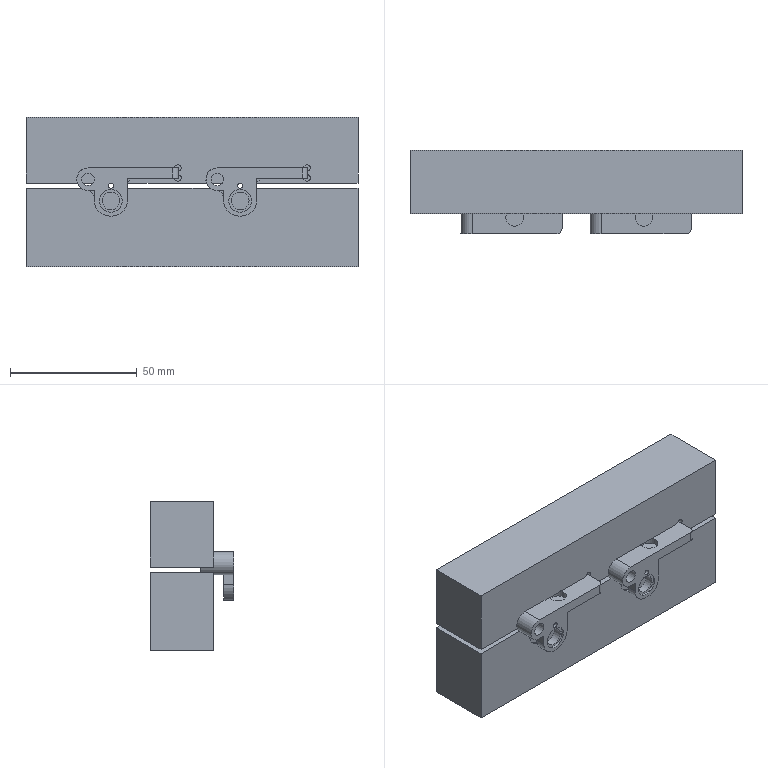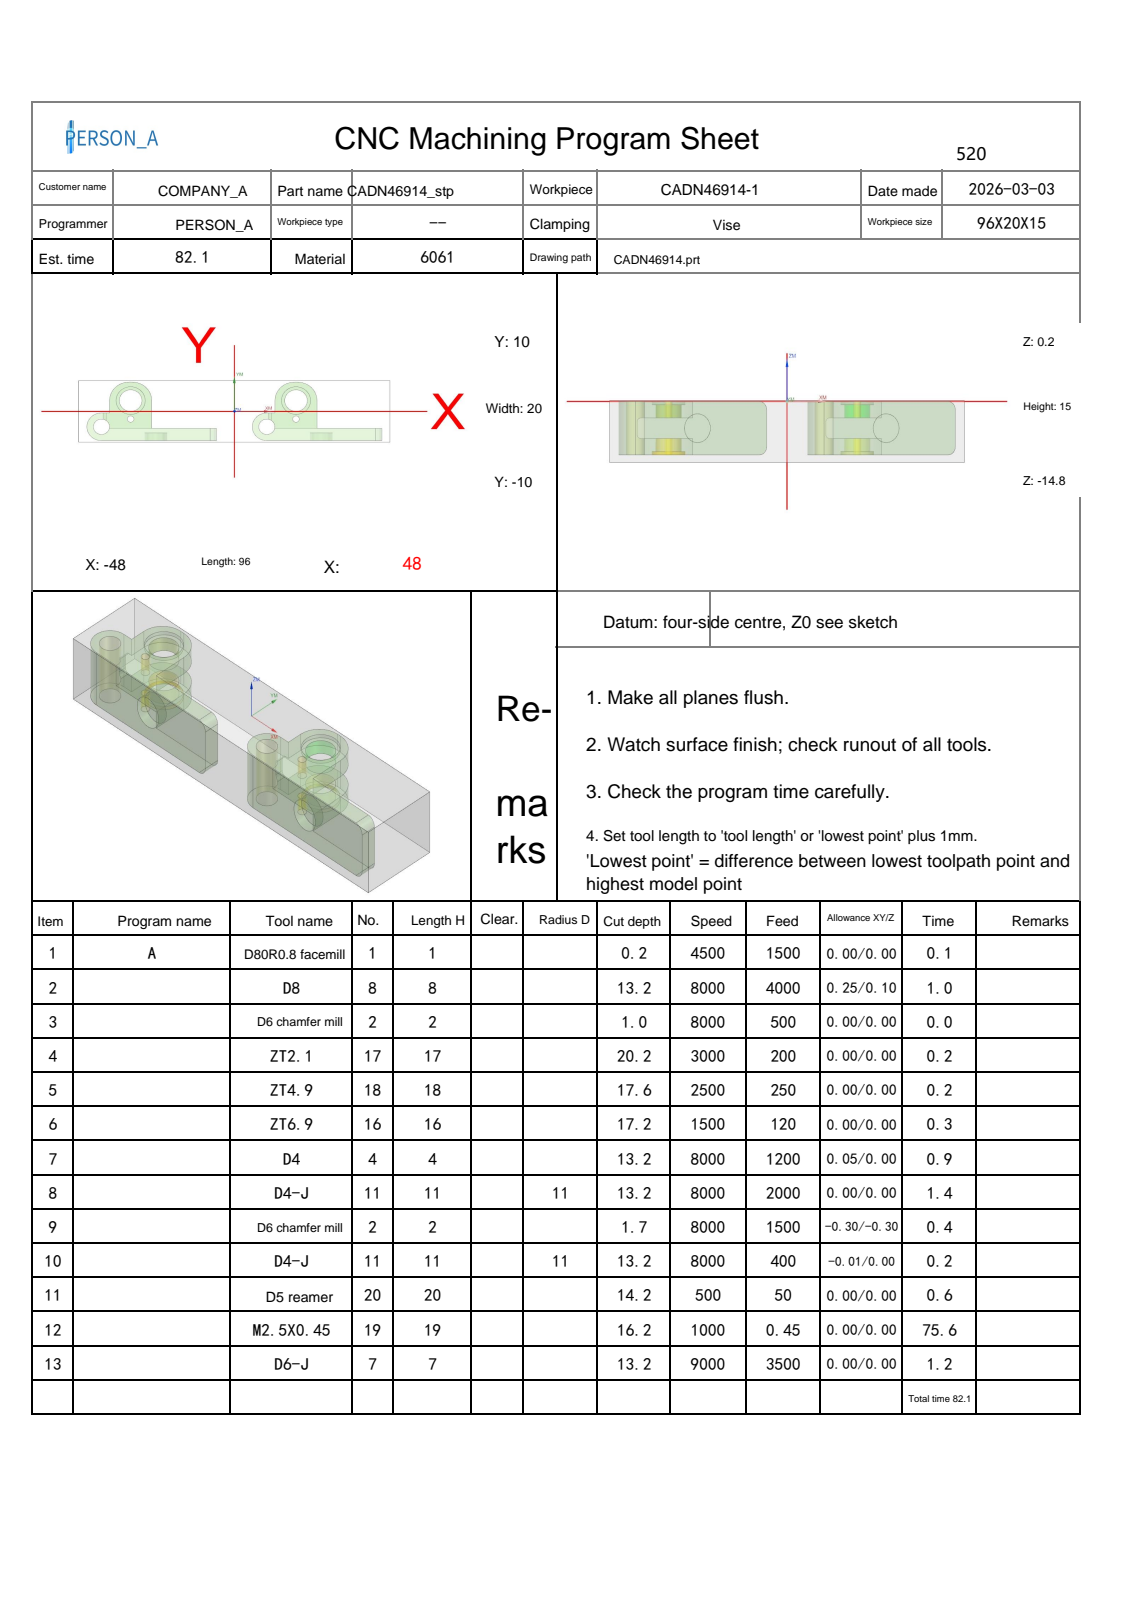NC program | NX | posted by the shop | part box 131 x 33 x 59 mm
Lines 1 to 1880 of 12027, first 1516 of 1878 lines:
%
O0001
(Machine time: 155.85 MIN)
(===Total Tool:11===)
(T1=D80R0.8 facemill D=80.  R=0.8  D-  H01 Z=-0.   )
(T8=D8      D=8.   R=0.   D-  H08 Z=-13.  )
(T2=D6 chamfer mill   D=6.   R=0.   D-  H02 Z=-1.5  )
(T17=ZT2.1  D=2.1  DR_a=118 D-  H17 Z=-20.  )
(T18=ZT4.9  D=4.9  DR_a=120 D-  H18 Z=-17.41)
(T16=ZT6.9  D=6.9  DR_a=120 D-  H16 Z=-17.  )
(T4=D4      D=4.   R=0.   D-  H04 Z=-13.  )
(T11=D4-J   D=4.   R=0.   D11 H11 Z=-13.  )
(T20=D5 reamer   D=5.   DR_a=180 D20 H20 Z=-14.  )
(T19=M2.5X0.45 D=2.05 DR_a=180 D-  H19 Z=-16.  )
(T7=D6-J    D=6.   R=0.   D7  H07 Z=-13.  )
G80 G90 G17 G49 G40
G91 G28 Z0
M01
N1 T01 M06
(D80R0.8 facemill  D=80. R=0.8 H=01 ce=0.00 di=0.00)
G00 G90 G54 X90.5 Y0.0 M03 S4500
G43 H01 Z50.
M08
Z2.
G01 Z0.0 F1500.
X85.5
X-85.5
X-90.5
Z2.
G00 Z50.
G91 G28 Z0.0
M05
M09
G91 G28 Z0.0
M01
N2 T08 M06
(D8  D=8. R=0. H=08 ce=0.25 di=0.10)
G00 G90 G54 X-31.173 Y-19.977 M03 S8000
G43 H08 Z50.
M08
Z-11.
G01 X-31.188 Y-19.879 Z-11.625 F4000.
X-31.204 Y-19.78 Z-11.872
X-31.219 Y-19.681 Z-12.054
X-31.234 Y-19.582 Z-12.2
X-31.249 Y-19.483 Z-12.323
X-31.265 Y-19.384 Z-12.428
X-31.28 Y-19.286 Z-12.52
X-31.295 Y-19.187 Z-12.6
X-31.31 Y-19.088 Z-12.67
X-31.326 Y-18.989 Z-12.732
X-31.341 Y-18.89 Z-12.786
X-31.356 Y-18.792 Z-12.833
X-31.372 Y-18.693 Z-12.874
X-31.387 Y-18.594 Z-12.908
X-31.402 Y-18.495 Z-12.936
X-31.417 Y-18.396 Z-12.96
X-31.433 Y-18.297 Z-12.977
X-31.448 Y-18.199 Z-12.99
X-31.463 Y-18.1 Z-12.997
X-31.478 Y-18.001 Z-13.
X-31.735 Y-16.34
G03 X-32.01 Y-16.017 I-.404 J-.066
X-35.519 Y-15.492 I-3.509 J-11.46
G01 X-35.593
G03 X-46.075 Y-15.381 I-10.483 J-496.321
G01 X-46.658 Y-15.382
G02 X-52.576 Y-10.87 I.001 J6.139
X-53.33 Y-5.373 I19.659 J5.497
G01 Y-5.3
G02 X-53.415 Y2.659 I373.963 J7.959
X-53.361 Y8.999 I374.048 J0.0
X-48.906 Y14.573 I6.101 J-.308
X-43.489 Y15.327 I5.418 J-19.103
G01 X-43.457 Y15.326
G02 X-34.113 Y15.4 I9.343 J-593.749
G01 X-33.498
X46.622 Y15.383
X46.677
G02 X52.525 Y11.02 I0.0 J-6.1
X53.318 Y5.638 I-18.167 J-5.425
X53.416 Y-2.714 I-356.305 J-8.352
X53.36 Y-9.02 I-356.403 J0.0
X49.041 Y-14.518 I-6.055 J.311
X43.556 Y-15.322 I-5.485 J18.317
G01 X43.54
G02 X34.581 Y-15.401 I-8.958 J507.142
G01 X33.58 Y-15.4
X-29.919 Y-15.386
G03 X-37.675 Y-14.858 I-12.074 J-120.03
G02 X-45.7 Y-14.758 I4.706 J700.045
X-51.384 Y-10.731 I.412 J6.606
X-52.632 Y-4.958 I14.903 J6.245
X-52.809 Y3.144 I185.372 J8.102
X-52.752 Y7.758 I185.549 J0.0
X-48.584 Y13.457 I6.632 J-.476
X-42.856 Y14.641 I6.186 J-15.48
X-34.645 Y14.811 I8.211 J-197.481
X-32.419 Y14.799 I0.0 J-197.652
G01 X45.361 Y14.777
G02 X51.385 Y10.727 I-.09 J-6.639
X52.62 Y5.134 I-14.626 J-6.161
X52.813 Y-3.12 I-176.538 J-8.254
X52.752 Y-7.761 I-176.731 J0.0
X48.731 Y-13.383 I-6.598 J.47
X43.199 Y-14.619 I-6.112 J14.36
X33.955 Y-14.822 I-9.244 J209.879
X30.842 Y-14.799 I0.0 J210.083
G01 X-28.817 Y-14.779
G03 X-38.511 Y-14.261 I-20.809 J-298.283
G01 X-38.8
G02 X-44.696 Y-14.139 I0.0 J142.819
X-50.671 Y-9.697 I.775 J7.281
X-51.996 Y-3.753 I15.854 J6.653
X-52.209 Y2.694 I97.671 J6.447
X-52.125 Y6.741 I97.884 J0.0
X-47.707 Y12.669 I7.254 J-.796
X-41.584 Y14.01 I6.722 J-16.049
X-31.957 Y14.222 I9.626 J-217.839
X-29.047 Y14.203 I0.0 J-218.052
G01 X44.038 Y14.178
G02 X50.697 Y9.638 I-.131 J-7.345
X52.001 Y3.691 I-16.077 J-6.639
X52.205 Y-2.78 I-102.305 J-6.471
X52.131 Y-6.684 I-102.51 J0.0
X48.862 Y-12.04 I-7.112 J.664
X47.625 Y-13.181 I-3.464 J2.517
X45.5 Y-13.75 I-2.305 J4.352
X36.302 Y-14.202 I-9.198 J93.33
X34.835 Y-14.191 I0.0 J93.782
G01 X-27.645 Y-14.182
G02 X-36.111 Y-13.75 I31.277 J696.242
X-38.142 Y-13.775 I-2.03 J82.632
X-42.93 Y-13.636 I0.0 J82.657
X-50.092 Y-8.528 I.327 J8.034
X-51.415 Y-2.034 I18.291 J7.107
X-51.579 Y2.607 I65.409 J4.64
X-51.514 Y5.521 I65.573 J0.0
X-46.754 Y11.985 I7.803 J-.761
X-40.64 Y13.371 I6.966 J-16.556
X-34.235 Y13.583 I6.881 J-110.809
X-31.707 Y13.747 I2.528 J-19.451
X-29.968 Y13.67 I0.0 J-19.614
G03 X-20.778 Y13.6 I9.191 J605.473
G01 X-20.602
X16.938
G02 X19.516 Y13.752 I2.578 J-21.824
X21.449 Y13.666 I0.0 J-21.976
G03 X34.707 Y13.576 I13.258 J972.338
X41.458 Y13.599 I0.0 J972.429
G02 X42.084 Y13.617 I.626 J-10.91
X45.763 Y12.979 I0.0 J-10.928
X50.312 Y7.97 I-3.406 J-7.663
X51.448 Y1.494 I-20.828 J-6.991
X51.582 Y-2.563 I-61.296 J-4.057
X51.507 Y-5.581 I-61.431 J0.0
X49.714 Y-9.906 I-8.423 J.958
X48.852 Y-12.053 I-3.864 J.305
G03 X49.706 Y-9.872 I-2.976 J2.423
X51.03 Y-2.986 I-17.238 J6.886
X51.026 Y-2.565 I-18.562 J0.0
X51.047 Y-1.316 I-37.014 J1.249
X50.415 Y5.496 I-37.035 J0.0
X47.669 Y10.726 I-9.664 J-1.738
X42.536 Y12.852 I-5.851 J-6.867
X36.521 Y13.127 I-6.015 J-65.771
X35.284 Y13.115 I0.0 J-66.046
G02 X32.132 Y13.106 I-3.152 J555.883
X22.821 Y13.184 I0.0 J555.892
G03 X20.121 Y13.728 I-3.812 J-11.937
G02 X23.466 Y12.961 I-1.169 J-12.769
G03 X28.086 Y12.551 I4.62 J25.827
X28.536 Y12.555 I0.0 J26.237
G01 X28.787
G02 X39.905 Y12.42 I0.0 J-457.028
X44.815 Y11.431 I-.102 J-13.192
X49.287 Y6.166 I-3.935 J-7.873
X50.357 Y-.852 I-22.46 J-7.018
G01 Y-.865
G02 X50.391 Y-2.083 I-22.145 J-1.218
X49.75 Y-7.376 I-22.178 J0.0
X49.771 Y-8.246 I-17.879 J-.87
X49.687 Y-9.978 I-17.9 J0.0
G03 X49.771 Y-8.246 I-17.816 J1.731
X49.75 Y-7.376 I-17.9 J0.0
G01 X49.856 Y-1.619
G03 X49.859 Y-1.299 I-23.764 J.32
X48.904 Y5.37 I-23.766 J0.0
X42.148 Y11.442 I-8.36 J-2.507
X35.985 Y12.016 I-6.163 J-32.851
X35.464 Y12.012 I0.0 J-33.424
G02 X34.223 Y12.007 I-1.241 J169.499
X25.721 Y12.22 I0.0 J169.503
X24.568 Y12.388 I.85 J9.879
G03 X22.994 Y13.11 I-4.602 J-7.962
G02 X25.036 Y12.15 I-7.062 J-17.675
G03 X29.128 Y11.549 I4.183 J14.252
G02 X38.003 Y11.306 I-17.561 J-803.143
X43.381 Y10.202 I-.355 J-15.383
X48.148 Y4.731 I-3.889 J-8.2
X49.199 Y-2.119 I-21.803 J-6.85
X49.192 Y-2.663 I-22.854 J0.0
G01 X49.213 Y-3.454
G02 X49.75 Y-5.502 I-4.134 J-2.177
G01 Y-6.282
G03 X49.77 Y-5.816 I-5.325 J.466
X49.181 Y-3.375 I-5.345 J0.0
G02 X48.598 Y.165 I21.975 J5.431
G03 X46.88 Y5.94 I-15.451 J-1.456
X40.825 Y10.245 I-7.949 J-4.77
X34.296 Y10.925 I-6.529 J-31.005
G01 X34.213
X34.11
G02 X26.951 Y11.311 I0.0 J66.524
G01 X25.816 Y11.561
X24.666 Y12.323
G03 X26.591 Y11.159 I6.474 J8.534
X31.008 Y10.477 I4.736 J16.027
G02 X38.201 Y10.026 I-2.816 J-102.487
X43.722 Y8.015 I-1.074 J-11.533
X47.372 Y2.285 I-6.546 J-8.197
X48.355 Y-2.273 I-119.995 J-28.268
G01 X49.181 Y-3.375
G02 X48.159 Y-1.981 I6.846 J6.089
X46.987 Y1.793 I41.138 J14.841
G03 X43.528 Y7.177 I-10.292 J-2.81
X37.723 Y9.457 I-7.253 J-9.935
X30.746 Y10.029 I-11.086 J-92.462
G02 X26.669 Y10.791 I.523 J14.084
G01 X25.902 Y11.504
G03 X27.46 Y10.29 I3.757 J3.213
X31.921 Y9.416 I5.217 J14.815
G02 X38.256 Y8.659 I-2.824 J-50.506
X45.91 Y2.299 I-1.91 J-10.083
G03 X47.389 Y-1.48 I172.833 J65.472
X47.654 Y-1.842 I1.213 J.612
G01 X48.505 Y-2.495
G02 X47.254 Y-1.443 I3.601 J5.554
X45.612 Y1.782 I20.773 J12.61
G03 X37.889 Y8.06 I-9.997 J-4.408
X31.486 Y8.985 I-10.718 J-51.591
G02 X27.474 Y9.945 I1.011 J13.082
G01 X26.707 Y10.733
X27.657 Y9.749
G03 X30.84 Y8.612 I4.25 J6.871
G02 X36.544 Y7.677 I-31.05 J-207.346
X42.97 Y4.191 I-2.042 J-11.431
X45.724 Y-.006 I-17.256 J-14.325
G03 X46.785 Y-1.471 I4.78 J2.344
G01 X47.625 Y-1.819
G02 X45.51 Y-.187 I.987 J3.466
G03 X42.711 Y3.573 I-27.418 J-17.488
X36.083 Y7.146 I-9.148 J-9.038
X30.559 Y8.223 I-147.226 J-740.215
G02 X27.945 Y9.244 I1.369 J7.362
G01 X27.382 Y10.021
G03 X28.579 Y8.664 I3.988 J2.314
X32.273 Y7.366 I5.699 J10.306
G02 X37.757 Y5.902 I-6.117 J-33.935
X43.459 Y1.443 I-5.166 J-12.481
G03 X45.783 Y-1.221 I14.294 J10.126
X46.552 Y-1.395 I.769 J1.603
G01 X46.6
X46.766 Y-1.464
G03 X45.858 Y-1.291 I-1.165 J-3.644
G02 X44.043 Y.177 I2.657 J5.141
G03 X40.286 Y3.777 I-18.712 J-15.769
X34.18 Y6.38 I-9.926 J-14.824
G02 X29.59 Y7.744 I6.19 J29.231
X28.444 Y8.458 I1.201 J3.205
G03 X27.987 Y9.186 I-4.09 J-2.058
G02 X28.589 Y8.228 I-8.375 J-5.928
G03 X31.202 Y6.722 I4.379 J4.577
G02 X36.446 Y4.995 I-38.225 J-124.917
X42.373 Y.943 I-6.601 J-16.016
G03 X44.889 Y-1.205 I10.39 J9.625
X45.918 Y-1.305 I1.921 J14.366
G01 X44.785 Y-1.206
G02 X42.289 Y.489 I3.565 J7.938
G03 X33.8 Y5.338 I-14.658 J-15.807
G02 X29.642 Y7.011 I6.022 J20.969
X28.838 Y7.638 I3.077 J4.776
G01 X28.448 Y8.449
G03 X30.515 Y6.173 I3.713 J1.295
X35.12 Y4.219 I22.525 J46.705
G02 X41.577 Y.243 I-10.156 J-23.721
G03 X43.934 Y-1.25 I5.877 J6.67
G01 X45.014
G02 X44.527 Y-1.274 I-.487 J4.881
X43.37 Y-1.136 I0.0 J4.905
X40.919 Y.26 I4.622 J10.961
G03 X32.709 Y4.653 I-21.189 J-29.733
G02 X29.437 Y6.505 I4.235 J11.296
X29.099 Y7.095 I.544 J.705
G01 X28.865 Y7.581
G02 X29.269 Y6.587 I-9.624 J-4.486
G03 X31.573 Y4.706 I4.861 J3.604
G02 X36.73 Y2.126 I-209.579 J-425.324
X41.434 Y-.747 I-161.623 J-269.946
G03 X42.527 Y-1.25 I5.588 J10.704
G01 X43.907
G02 X43.306 Y-1.268 I-.601 J10.276
X42.088 Y-1.195 I0.0 J10.293
X39.12 Y.202 I3.955 J12.253
G03 X32.066 Y3.936 I-66.016 J-116.184
G02 X29.431 Y5.933 I3.5 J7.356
G01 X29.178 Y6.806
G03 X30.83 Y4.273 I3.652 J.577
X35.517 Y1.522 I21.392 J31.078
X40.498 Y-1.128 I34.794 J59.372
G01 X40.859 Y-1.25
X42.419
G02 X41.73 Y-1.271 I-.689 J11.345
X40.269 Y-1.177 I0.0 J11.366
X36.368 Y.546 I5.797 J18.405
X30.985 Y3.673 I18.062 J37.293
X29.621 Y5.075 I3.161 J4.437
G01 X29.427 Y5.904
G03 X29.718 Y4.751 I17.361 J3.776
X31.989 Y2.469 I5.796 J3.497
X38.937 Y-1.245 I20.168 J29.377
G01 X40.768 Y-1.25
G02 X39.994 Y-1.268 I-.775 J16.568
X38.383 Y-1.19 I0.0 J16.586
X34.006 Y.714 I4.674 J16.724
X30.252 Y3.475 I6.689 J13.028
X29.673 Y4.353 I2.922 J2.557
G01 X29.603 Y5.13
X29.602 Y5.04
G03 X30.737 Y2.548 I3.303 J0.0
X36.993 Y-1.25 I12.111 J12.897
G01 X38.853
G02 X38.008 Y-1.275 I-.845 J14.422
X36.336 Y-1.178 I0.0 J14.446
X30.251 Y2.605 I3.331 J12.143
X29.75 Y3.499 I1.575 J1.471
G01 X29.68 Y4.276
X29.679 Y4.187
G03 X29.98 Y2.679 I3.927 J0.0
X32.983 Y-.206 I7.071 J4.355
X35.145 Y-1.25 I5.901 J9.46
G01 X36.825
G02 X36.086 Y-1.272 I-.739 J12.686
X34.564 Y-1.18 I0.0 J12.707
X29.937 Y2.206 I2.125 J7.756
G01 X29.75 Y2.657
Y3.437
G03 X29.726 Y3.046 I3.189 J-.392
X30.742 Y.701 I3.213 J0.0
X33.598 Y-1.25 I5.495 J4.978
G01 X35.038
G02 X34.41 Y-1.27 I-.629 J9.936
X33.153 Y-1.19 I0.0 J9.956
X29.759 Y1.732 I1.504 J5.178
G01 X29.75 Y2.574
G03 X29.725 Y2.182 I3.114 J-.392
X30.825 Y-.204 I3.139 J0.0
X32.422 Y-1.25 I3.235 J3.196
G01 X33.562
G02 X33.052 Y-1.274 I-.51 J5.425
X31.971 Y-1.166 I0.0 J5.449
X29.75 Y.99 I1.21 J3.469
G01 Y1.71
G03 X29.726 Y1.345 I2.716 J-.365
X30.054 Y.044 I2.74 J0.0
X31.564 Y-1.25 I2.586 J1.489
G01 X32.404
G02 X32.017 Y-1.274 I-.386 J3.127
X31.124 Y-1.145 I0.0 J3.151
X29.75 Y.312 I1.012 J2.332
G01 Y.912
G03 X29.726 Y.6 I2.005 J-.313
X30.892 Y-1.237 I2.029 J0.0
G01 X31.505 Y-1.25
G02 X31.239 Y-1.273 I-.266 J1.543
X29.75 Y-.189 I0.0 J1.565
G01 Y.231
G03 X29.726 Y-.02 I1.309 J-.251
X30.529 Y-1.242 I1.333 J0.0
G01 X30.935 Y-1.25
G02 X30.717 Y-1.275 I-.218 J.946
X29.745 Y-.304 I0.0 J.971
G01 X29.75 Y-.209
G03 X29.727 Y-.41 I.871 J-.202
X30.313 Y-1.25 I.894 J0.0
G01 X30.553
X30.404 Y-1.267
G02 X29.743 Y-.606 I0.0 J.661
G01 X29.75 Y-.513
X29.736 Y-.648
G03 X29.991 Y-1.161 I.642 J0.0
X30.247 Y-1.243 I.256 J.359
X30.688 Y-.802 I0.0 J.441
X30.28 Y-.363 I-.441 J0.0
G01 X30.205 Y-.356
G03 X29.765 Y-.797 I0.0 J-.44
G01 X29.774 Y-.883
G03 X30.264 Y-1.258 I.491 J.134
G01 X30.355 Y-1.25
G03 X30.71 Y-1.033 I-.003 J.405
G01 X30.999 Y-.471
X31.721 Y.933 Z-12.9
X32.086 Y1.643
X32.111 Y1.702
X32.126 Y1.763
X32.131 Y1.826
Y4.787
X32.126 Y5.067
X32.11 Y5.347
X32.085 Y5.626
X32.049 Y5.904
X32.003 Y6.181
X31.947 Y6.456
X31.881 Y6.728
X31.794 Y7.044
X31.696 Y7.357
X31.588 Y7.667
X31.471 Y7.973
X31.345 Y8.276
X31.209 Y8.574
X31.063 Y8.868
X30.909 Y9.157
X30.745 Y9.441
X30.571 Y9.719
X30.389 Y9.992
X30.198 Y10.258
X29.611 Y11.051
X29.373 Y11.363
X29.127 Y11.669
X28.873 Y11.968
X28.611 Y12.259
X28.341 Y12.544
X28.063 Y12.822
X27.779 Y13.091
X27.487 Y13.353
X27.188 Y13.608
X26.882 Y13.854
X25.662 Y14.809
X25.447 Y14.97
X25.226 Y15.123
X24.999 Y15.266
X24.767 Y15.4
X24.529 Y15.524
X24.286 Y15.639
X24.039 Y15.744
X23.788 Y15.838
X23.533 Y15.923
X23.275 Y15.997
X23.014 Y16.06
X22.751 Y16.113
X22.485 Y16.155
X18.714 Y16.676
X18.648 Y16.68
X18.582 Y16.672
X18.518 Y16.654
X18.458 Y16.625
X18.403 Y16.587
X18.356 Y16.54
X18.317 Y16.486
X18.287 Y16.427
X18.003 Y15.706
X17.424 Y14.237 Z-13.
X17.329 Y13.985
G02 X16.938 Y13.6 I-.492 J.109
G01 X15.149 Y13.304
G02 X8.743 Y13.107 I-6.405 J103.748
X7.014 Y13.121 I0.0 J103.946
G01 X-27.558 Y13.149
X-28.231 Y13.167
X-29.458 Y13.544
X-31.428 Y13.743
X-29.458 Y13.544
G03 X-24.297 Y12.607 I5.246 J14.21
X-15.735 Y12.518 I8.561 J410.51
X-14.362 Y12.52 I0.0 J410.6
G01 X10.788 Y12.544
G03 X14.055 Y12.688 I-.372 J45.413
G01 X14.667 Y13.006
X16.336 Y13.499
X14.667 Y13.006
G02 X11.781 Y12.219 I-2.985 J5.261
X4.783 Y12.026 I-6.998 J126.839
X2.875 Y12.041 I0.0 J127.032
G01 X-21.55 Y12.068
G02 X-21.897 Y12.066 I-.347 J33.782
X-26.47 Y12.377 I0.0 J33.783
G01 X-27.601 Y12.973
G03 X-25.595 Y12.017 I6.158 J10.339
X-20.887 Y11.507 I4.708 J21.485
G01 X-20.8 Y11.508
X-13.701 Y11.441
X7.544 Y11.467
G03 X7.906 Y11.465 I.362 J31.589
X12.512 Y11.803 I0.0 J31.591
G02 X14.044 Y12.682 I4.837 J-6.65
G03 X12.379 Y11.713 I4.424 J-9.511
G02 X8.667 Y11.086 I-3.764 J10.979
X.68 Y10.952 I-7.987 J238.625
X-1.384 Y10.961 I0.0 J238.758
X-7.365 Y10.941 I-5.982 J888.77
X-20.757 Y11.042 I0.0 J888.791
X-25.198 Y11.549 I.125 J20.788
G03 X-26.308 Y12.29 I-3.467 J-3.993
G02 X-25.065 Y11.436 I-2.759 J-5.349
G03 X-21.79 Y10.623 I3.716 J7.971
X-14.513 Y10.355 I7.277 J98.441
X-13.157 Y10.364 I0.0 J98.71
X-6.312 Y10.336 I6.844 J845.53
X7.286 Y10.446 I0.0 J845.558
X11.495 Y10.975 I-.047 J17.371
G01 X12.568 Y11.818
G02 X10.99 Y10.696 I-4.898 J5.218
X6.867 Y10.016 I-4.309 J13.3
X-1.592 Y9.869 I-8.459 J243.937
X-3.964 Y9.881 I0.0 J244.084
X-8.424 Y9.857 I-4.46 J418.489
X-19.454 Y10.003 I0.0 J418.512
X-24.197 Y10.716 I.16 J17.197
G01 X-25.233 Y11.554
G03 X-23.576 Y10.319 I5.751 J5.99
X-19.261 Y9.48 I4.731 J12.814
X-10.459 Y9.265 I8.802 J179.664
X-8.001 Y9.281 I0.0 J179.88
X-3.994 Y9.258 I4.007 J338.584
X6.331 Y9.415 I0.0 J338.608
X10.699 Y10.151 I-.186 J14.434
X11.389 Y10.882 I-1.834 J2.423
G01 X11.53 Y10.993
X10.641 Y10.066
G02 X7.445 Y9.132 I-3.732 J6.835
X-.038 Y8.792 I-7.483 J82.287
X-1.511 Y8.805 I0.0 J82.627
X-6.287 Y8.78 I-4.776 J443.435
X-17.6 Y8.924 I0.0 J443.461
X-22.796 Y9.664 I.259 J20.419
X-23.706 Y10.083 I2.345 J6.299
G01 X-24.234 Y10.73
G03 X-21.627 Y8.994 I3.374 J2.242
X-15.794 Y8.302 I6.053 J26.069
X-6.195 Y8.179 I9.599 J374.951
X4.661 Y8.336 I0.0 J375.074
X9.619 Y9.133 I-.211 J17.13
X10.112 Y9.391 I-1.091 J2.684
G01 X10.815 Y10.211
G02 X9.707 Y9.053 I-4.568 J3.258
X6.092 Y8.057 I-4.272 J8.447
X-2.061 Y7.709 I-8.153 J95.281
X-3.788 Y7.724 I0.0 J95.629
X-7.113 Y7.702 I-3.325 J243.003
X-17.007 Y7.903 I0.0 J243.026
X-22.265 Y8.834 I.452 J17.866
G01 X-22.995 Y9.212
X-23.64 Y10.002
G03 X-22.361 Y8.672 I4.384 J2.934
X-18.394 Y7.532 I4.859 J9.437
X-10.509 Y7.13 I7.885 J77.167
X-9.602 Y7.135 I0.0 J77.569
X-5.66 Y7.101 I3.942 J226.131
X4.015 Y7.308 I0.0 J226.165
X8.932 Y8.226 I-.438 J15.966
X9.72 Y8.7 I-1.066 J2.665
G01 X10.112 Y9.391
G02 X8.33 Y7.758 I-2.608 J1.057
X3.175 Y6.832 I-5.63 J16.523
X-6.15 Y6.622 I-9.325 J206.845
X-16.139 Y6.863 I0.0 J207.055
X-21.427 Y7.854 I.672 J18.192
X-22.649 Y8.582 I1.375 J3.697
G01 X-22.967 Y9.178
G03 X-20.997 Y7.361 I2.944 J1.215
X-15.643 Y6.296 I6.125 J16.806
X-5.948 Y6.029 I9.695 J175.564
X3.264 Y6.27 I0.0 J175.831
X8.352 Y7.305 I-.615 J16.056
X9.238 Y7.852 I-1.335 J3.152
G01 X9.712 Y8.686
G02 X8.957 Y7.521 I-4.081 J1.819
X5.727 Y6.208 I-4.284 J5.907
X-1.719 Y5.603 I-7.446 J45.529
X-2.101 Y5.605 I0.0 J46.134
X-6.175 Y5.55 I-4.073 J150.116
X-15.725 Y5.854 I0.0 J150.171
X-21.063 Y7.017 I.866 J16.797
X-22.213 Y7.763 I1.879 J4.16
G01 X-22.608 Y8.504
G03 X-20.464 Y6.423 I3.359 J1.316
X-15.175 Y5.279 I6.315 J16.394
X-6.019 Y4.96 I9.156 J131.247
X2.91 Y5.263 I0.0 J131.566
X7.876 Y6.396 I-.875 J15.281
X8.973 Y7.179 I-.966 J2.515
G01 X9.232 Y7.841
X8.929 Y7.068
G02 X6.686 Y5.634 I-3.425 J2.886
X.908 Y4.683 I-6.486 J21.373
X-6.014 Y4.489 I-6.922 J123.716
X-15.04 Y4.818 I0.0 J123.91
X-20.462 Y6.044 I1.06 J17.291
X-21.899 Y7.028 I1.783 J4.145
G03 X-22.166 Y7.674 I-7.638 J-2.785
G02 X-21.821 Y6.85 I-17.117 J-7.649
G03 X-19.394 Y5.231 I3.846 J3.135
X-13.216 Y4.129 I7.12 J22.056
X-6.176 Y3.903 I7.041 J109.829
X2.286 Y4.229 I0.0 J110.054
X7.478 Y5.488 I-1.001 J15.466
X8.714 Y6.409 I-1.257 J2.977
G01 X8.963 Y7.148
G02 X7.402 Y5.195 I-2.649 J.518
X2.429 Y3.835 I-6.104 J12.545
X-6.247 Y3.43 I-8.676 J92.766
X-10.326 Y3.52 I0.0 J93.171
X-18.038 Y4.403 I.292 J36.673
X-21.477 Y6.082 I1.594 J7.625
G01 X-21.714 Y6.38
X-21.922 Y7.069
G03 X-20.273 Y4.896 I2.953 J.528
X-15.23 Y3.367 I6.498 J12.349
X-6.272 Y2.848 I8.958 J77.036
X-3.572 Y2.895 I0.0 J77.555
G01 X-3.352 Y2.894
G03 X4.593 Y3.674 I0.0 J40.894
X8.17 Y5.267 I-1.594 J8.39
X8.517 Y5.825 I-.435 J.657
G01 X8.69 Y6.337
G02 X8.399 Y5.428 I-10.65 J2.905
X5.961 Y3.749 I-3.942 J3.113
X-.491 Y2.577 I-7.254 J21.587
X-6.032 Y2.386 I-5.541 J80.28
X-14.684 Y2.852 I0.0 J80.471
X-20.009 Y4.362 I1.506 J15.452
X-21.469 Y5.57 I1.89 J3.772
G01 X-21.695 Y6.317
G03 X-20.052 Y4.038 I3.155 J.543
X-14.94 Y2.378 I6.737 J12.041
X-6.109 Y1.804 I8.831 J67.731
X-2.877 Y1.881 I0.0 J68.304
X4.73 Y2.83 I-.26 J33.056
X8.084 Y4.563 I-1.773 J7.54
X8.41 Y5.024 I-1.272 J1.248
G01 X8.498 Y5.679
Y5.66
G02 X7.466 Y3.801 I-2.19 J0.0
X3.04 Y2.05 I-6.079 J8.892
X-5.339 Y1.354 I-8.379 J50.094
X-6.644 Y1.37 I0.0 J50.79
X-7.377 Y1.365 I-.733 J47.927
X-16.118 Y2.169 I0.0 J47.933
X-20.49 Y3.965 I1.907 J10.859
X-21.399 Y5.018 I1.576 J2.28
G01 X-21.446 Y5.492
G03 X-20.468 Y3.628 I2.307 J.021
X-16.2 Y1.703 I6.239 J8.141
X-7.492 Y.803 I8.708 J41.664
X-7.174 Y.804 I0.0 J42.564
X-5.519 Y.777 I1.655 J50.755
X2.741 Y1.453 I0.0 J50.782
X4.772 Y2.001 I-2.124 J11.918
G02 X7.154 Y3.274 I6.193 J-8.721
G03 X8.322 Y4.361 I-.98 J2.223
G01 X8.409 Y5.015
X8.41 Y4.963
G02 X7.68 Y3.43 I-1.976 J0.0
G01 X6.756 Y3.092
G03 X7.971 Y3.58 I-1.042 J4.357
X8.324 Y4.264 I-.488 J.684
G01 X8.32 Y4.346
X8.323 Y4.268
G02 X8.042 Y3.582 I-.981 J0.0
X7.766 Y3.485 I-.276 J.347
X7.322 Y3.929 I0.0 J.444
X7.52 Y4.298 I.444 J0.0
X7.822 Y4.418 I.302 J-.32
X8.262 Y3.978 I0.0 J-.44
G01 X8.249 Y3.87
G02 X7.679 Y3.412 I-.645 J.219
G03 X4.54 Y1.829 I2.432 J-8.723
G02 X.888 Y.768 I-4.752 J9.544
X-6.206 Y.319 I-7.094 J55.901
X-14.78 Y.976 I0.0 J56.35
X-19.891 Y2.796 I1.958 J13.581
X-21.33 Y4.316 I1.932 J3.27
G01 X-21.395 Y4.973
Y4.916
G03 X-20.23 Y2.688 I2.712 J0.0
X-15.723 Y.676 I6.655 J8.851
X-6.858 Y-.239 I8.865 J42.477
X-5.797 Y-.226 I0.0 J43.392
X-5.09 Y-.233 I.706 J37.152
X2.257 Y.501 I0.0 J37.159
X3.598 Y.964 I-.785 J4.446
G01 X4.767 Y1.996
G02 X3.243 Y.686 I-11.47 J11.802
X-.444 Y-.343 I-4.652 J9.548
X-6.314 Y-.698 I-5.87 J48.296
X-14.941 Y.073 I0.0 J48.651
X-20.024 Y2.122 I2.122 J12.591
X-21.254 Y3.54 I2.18 J3.133
G01 X-21.319 Y4.197
Y4.159
G03 X-20.137 Y1.841 I2.863 J0.0
X-15.406 Y-.32 I7.004 J9.074
X-6.416 Y-1.261 I8.991 J42.508
X-4.11 Y-1.2 I0.0 J43.449
X1.925 Y-.345 I-.238 J23.414
X2.96 Y.129 I-1.364 J4.342
G01 X3.598 Y.964
G02 X2.629 Y-.173 I-4.422 J2.788
X-1.034 Y-1.339 I-4.541 J7.929
X-3.813 Y-1.585 I-2.779 J15.563
G01 X-3.932
G03 X-5.487 Y-1.25 I-1.649 J-3.884
G02 X-8.046 Y-1.275 I-2.558 J132.55
X-12.56 Y-1.198 I0.0 J132.574
X-19.238 Y.781 I1.041 J15.771
X-21.235 Y2.825 I2.358 J4.302
G01 X-21.25 Y3.499
G03 X-21.264 Y3.226 I2.574 J-.273
X-20.323 Y1.229 I2.589 J0.0
X-15.973 Y-1.062 I6.784 J7.605
G01 X-15.249 Y-1.25
X-11.649
G02 X-13.31 Y-1.274 I-1.661 J56.637
X-16.144 Y-1.204 I0.0 J56.661
X-20.866 Y1.43 I1.09 J7.504
X-21.25 Y2.171 I2.417 J1.723
G01 Y2.891
G03 X-21.274 Y2.524 I2.754 J-.368
X-20.278 Y.392 I2.778 J0.0
X-17.527 Y-1.25 I4.982 J5.221
G01 X-15.667
G02 X-16.463 Y-1.266 I-.796 J20.258
X-17.96 Y-1.21 I0.0 J20.273
X-21.234 Y1.318 I1.004 J4.683
G01 X-21.25 Y2.062
G03 X-21.269 Y1.746 I2.694 J-.317
X-20.182 Y-.426 I2.713 J0.0
X-18.812 Y-1.25 I2.753 J3.025
G01 X-17.612
G02 X-18.149 Y-1.273 I-.536 J6.205
X-19.251 Y-1.175 I0.0 J6.228
X-21.25 Y.699 I.975 J3.043
G01 Y1.299
G03 X-21.268 Y1.004 I2.355 J-.295
X-19.64 Y-1.25 I2.373 J0.0
G01 X-18.86
G02 X-19.22 Y-1.272 I-.361 J2.888
X-20.07 Y-1.146 I0.0 J2.911
X-21.25 Y.109 I.866 J1.997
G01 Y.589
G03 X-21.272 Y.318 I1.651 J-.272
X-20.184 Y-1.25 I1.673 J0.0
G01 X-19.644
G02 X-19.908 Y-1.275 I-.264 J1.395
X-21.25 Y-.317 I0.0 J1.42
G01 Y.103
G03 X-21.272 Y-.128 I1.218 J-.231
X-20.586 Y-1.237 I1.24 J0.0
G01 X-20.213 Y-1.25
G02 X-20.412 Y-1.274 I-.199 J.817
X-21.253 Y-.433 I0.0 J.841
G01 X-21.25 Y-.36
X-21.274 Y-.544
G03 X-20.57 Y-1.25 I.706 J0.0
G01 X-20.659 Y-1.257
G02 X-21.185 Y-.961 I0.0 J.615
X-21.244 Y-.741 I.381 J.22
X-20.804 Y-.301 I.44 J0.0
X-20.495 Y-.428 I0.0 J-.44
X-20.301 Y-.797 I-.253 J-.369
X-20.748 Y-1.245 I-.448 J0.0
G01 X-20.824 Y-1.238
G02 X-21.259 Y-.739 I.07 J.5
G01 X-21.25 Y-.645
G02 X-21.03 Y-.288 I.405 J-.003
G01 X-20.432 Y.012
X-19.021 Y.721 Z-12.9
X-18.732 Y.866
X-18.676 Y.889
X-18.618 Y.903
X-18.558 Y.909
X-5.486 Y1.107
X-5.419 Y1.102
X-5.353 Y1.086
X-5.292 Y1.06
X-5.235 Y1.023
X-5.186 Y.978
X-5.144 Y.925
X-5.113 Y.865
X-5.038 Y.693
X-4.413 Y-.756 Z-13.
X-4.117 Y-1.428
G03 X-3.127 Y-1.783 I.99 J1.204
G01 X-3.102
G03 X-2.056 Y-1.84 I1.045 J9.579
X2.285 Y-.806 I0.0 J9.636
X2.563 Y-.39 I-.982 J.957
G01 X2.927 Y.087
G03 X2.373 Y-.759 I3.272 J-2.748
G02 X-.241 Y-1.963 I-3.314 J3.758
X-1.949 Y-2.155 I-1.708 J7.506
X-3.001 Y-2.083 I0.0 J7.698
G03 X-3.868 Y-1.611 I-1.705 J-2.104
G02 X-2.847 Y-2.179 I-1.623 J-4.121
G03 X-1.181 Y-2.43 I1.666 J5.392
X2.039 Y-1.422 I0.0 J5.643
G01 X2.431 Y-.658
G02 X.619 Y-2.363 I-2.481 J.822
X-1.165 Y-2.704 I-1.784 J4.49
X-2.433 Y-2.534 I0.0 J4.832
G01 X-2.483 Y-2.501
G02 X-2.58 Y-2.226 I.344 J.276
X-2.36 Y-1.844 I.441 J0.0
G01 X-1.937 Y-1.711 Z-12.972
X-1.507 Y-1.605 Z-12.944
X-.837 Y-1.43 Z-12.9
X-.042 Y-1.222
X1.486 Y-.822 Z-13.
X1.654 Y-.789
G02 X2.098 Y-1.232 I0.0 J-.444
X2.053 Y-1.426 I-.444 J0.0
X.209 Y-2.733 I-2.478 J1.542
X-1.106 Y-2.963 I-1.315 J3.641
X-2.194 Y-2.807 I0.0 J3.871
G03 X-3.063 Y-2.053 I-5.073 J-4.968
G02 X-2.251 Y-2.799 I-1.316 J-2.249
G03 X-.773 Y-3.196 I1.478 J2.553
X.103 Y-3.063 I0.0 J2.95
X1.697 Y-2.239 I-.667 J3.246
G01 X2.022 Y-1.489
G03 X1.7 Y-2.27 I6.731 J-3.237
G02 X-.705 Y-3.398 I-2.405 J1.999
X-1.991 Y-3.122 I0.0 J3.127
G01 X-2.302 Y-2.738
G03 X-.719 Y-3.613 I1.583 J.995
X-.472 Y-3.597 I0.0 J1.87
X1.551 Y-2.756 I0.0 J2.853
G01 X1.736 Y-2.173
G02 X.531 Y-3.578 I-1.675 J.217
X-.507 Y-3.799 I-1.038 J2.319
X-1.733 Y-3.484 I0.0 J2.541
G01 X-2.037 Y-3.084
G03 X-.488 Y-3.999 I1.549 J.852
X-.185 Y-3.973 I0.0 J1.768
X1.418 Y-3.228 I-.048 J2.2
G01 X1.582 Y-2.694
G02 X.379 Y-4.022 I-1.534 J.181
X-.375 Y-4.159 I-.754 J2.013
X-1.636 Y-3.75 I0.0 J2.149
G01 X-1.812 Y-3.384
G03 X-.628 Y-4.303 I1.234 J.369
X-.227 Y-4.342 I.401 J2.023
X1.368 Y-3.587 I0.0 J2.063
G01 X1.447 Y-3.155
G02 X.511 Y-4.33 I-1.235 J.023
X-.277 Y-4.501 I-.788 J1.721
X-1.542 Y-4.016 I0.0 J1.893
G01 X-1.68 Y-3.702
G03 X-.368 Y-4.655 I1.313 J.427
G01 X-.244 Y-4.65
X-.075 Y-4.658
G03 X1.333 Y-3.908 I0.0 J1.697
G01 X1.398 Y-3.505
Y-3.511
G02 X.47 Y-4.671 I-1.189 J0.0
X-.205 Y-4.801 I-.675 J1.694
X-1.394 Y-4.36 I0.0 J1.824
G01 X-1.548 Y-4.021
G03 X-.263 Y-4.963 I1.285 J.406
G01 X-.091 Y-4.951
X-.011 Y-4.953
G03 X1.282 Y-4.266 I0.0 J1.56
G01 X1.342 Y-3.907
G02 X.404 Y-4.998 I-1.142 J.033
X-.164 Y-5.103 I-.568 J1.485
X-1.342 Y-4.582 I0.0 J1.59
G01 X-1.394 Y-4.392
G03 X-.567 Y-5.173 I.956 J.184
X-.053 Y-5.258 I.513 J1.502
X1.24 Y-4.591 I0.0 J1.587
G01 X1.294 Y-4.252
G02 X.405 Y-5.283 I-1.066 J.02
X-.117 Y-5.375 I-.523 J1.442
X-1.322 Y-4.791 I0.0 J1.534
G01 X-1.385 Y-4.461
G03 X-.525 Y-5.447 I1.023 J.024
X-.043 Y-5.523 I.482 J1.491
X1.24 Y-4.854 I0.0 J1.567
G01 X1.269 Y-4.43
X1.28 Y-4.578
G02 X.592 Y-5.49 I-.948 J0.0
X-.075 Y-5.643 I-.667 J1.377
X-1.291 Y-5.042 I0.0 J1.531
G01 X-1.352 Y-4.718
G03 X-.348 Y-5.746 I1.078 J.048
X.017 Y-5.794 I.365 J1.381
X1.256 Y-5.076 I0.0 J1.429
G01 X1.271 Y-4.686
X1.282 Y-4.836
G02 X.56 Y-5.772 I-.967 J0.0
X-.053 Y-5.901 I-.613 J1.394
X-1.249 Y-5.319 I0.0 J1.522
G01 X-1.317 Y-4.979
G03 X-.342 Y-6.004 I1.065 J.036
X.032 Y-6.054 I.374 J1.358
X1.259 Y-5.335 I0.0 J1.408
G01 X1.273 Y-4.949
X1.285 Y-5.1
G02 X.571 Y-6.034 I-.968 J0.0
X-.03 Y-6.16 I-.601 J1.362
X-1.22 Y-5.566 I0.0 J1.489
G01 X-1.283 Y-5.236
G03 X-.216 Y-6.277 I1.099 J.06
X.078 Y-6.31 I.294 J1.301
X1.266 Y-5.581 I0.0 J1.334
G01 X1.275 Y-5.211
X1.288 Y-5.368
G02 X.578 Y-6.291 I-.955 J0.0
X-.012 Y-6.419 I-.591 J1.307
X-1.226 Y-5.749 I0.0 J1.434
G01 X-1.25 Y-5.49
Y-5.517
G03 X-.491 Y-6.471 I.979 J0.0
X.042 Y-6.575 I.533 J1.309
X1.264 Y-5.87 I0.0 J1.413
G01 X1.278 Y-5.537
X1.284 Y-5.645
G02 X.598 Y-6.556 I-.948 J0.0
X.003 Y-6.687 I-.594 J1.286
X-1.233 Y-5.962 I0.0 J1.416
G01 X-1.25 Y-5.695
X-1.251 Y-5.742
G03 X-.358 Y-6.78 I1.05 J0.0
X.045 Y-6.838 I.402 J1.358
X1.302 Y-6.074 I0.0 J1.417
G01 X1.28 Y-5.717
G02 X1.308 Y-5.939 I-.854 J-.222
X.766 Y-6.753 I-.882 J0.0
X.013 Y-6.977 I-.754 J1.152
X-1.244 Y-6.164 I0.0 J1.377
G01 X-1.25 Y-5.886
X-1.254 Y-5.974
G03 X-.211 Y-7.09 I1.118 J0.0
X.08 Y-7.121 I.291 J1.343
X1.351 Y-6.27 I0.0 J1.374
G01 X1.305 Y-5.865
G02 X1.349 Y-6.158 I-.946 J-.292
X.651 Y-7.104 I-.99 J0.0
X.025 Y-7.252 I-.626 J1.249
X-1.241 Y-6.447 I0.0 J1.397
G01 X-1.25 Y-6.153
X-1.253 Y-6.241
G03 X-.131 Y-7.384 I1.143 J0.0
X.09 Y-7.402 I.221 J1.386
X1.393 Y-6.521 I0.0 J1.404
G01 X1.347 Y-6.114
G02 X1.39 Y-6.41 I-.996 J-.296
X.63 Y-7.411 I-1.039 J0.0
X.035 Y-7.544 I-.596 J1.27
X-1.243 Y-6.72 I0.0 J1.403
G01 X-1.25 Y-6.436
X-1.254 Y-6.527
G03 X-.159 Y-7.669 I1.144 J0.0
X.133 Y-7.701 I.292 J1.346
X1.442 Y-6.751 I0.0 J1.377
G01 X1.393 Y-6.381
G02 X1.437 Y-6.683 I-1.018 J-.302
X.648 Y-7.709 I-1.062 J0.0
X.062 Y-7.833 I-.586 J1.322
X-1.239 Y-7.018 I0.0 J1.446
G01 X-1.25 Y-6.711
X-1.254 Y-6.805
G03 X-.127 Y-7.968 I1.164 J0.0
X.156 Y-7.997 I.283 J1.383
X1.49 Y-7.045 I0.0 J1.412
G01 X1.452 Y-6.727
G02 X1.482 Y-6.978 I-1.022 J-.251
X.73 Y-7.987 I-1.053 J0.0
X.088 Y-8.132 I-.642 J1.348
X-1.237 Y-7.329 I0.0 J1.493
G01 X-1.25 Y-6.954
X-1.259 Y-7.099
G03 X-.149 Y-8.267 I1.169 J0.0
X.153 Y-8.298 I.302 J1.459
X1.537 Y-7.359 I0.0 J1.49
G01 X1.483 Y-6.913
G02 X1.537 Y-7.336 I-1.638 J-.423
X1.441 Y-7.897 I-1.691 J0.0
G03 X1.425 Y-8.271 I4.33 J-.374
X3.29 Y-11.839 I4.346 J0.0
X7.946 Y-13.477 I5.298 J7.62
G01 X8.268 Y-13.577
X9.999 Y-13.75
X45.5
G02 X45.9 Y-14.15 I0.0 J-.4
X45.715 Y-14.488 I-.4 J0.0
G01 X45.117 Y-14.867
X43.784 Y-15.714 Z-12.9
X43.514 Y-15.885
X43.465 Y-15.912
X43.412 Y-15.932
X43.358 Y-15.944
X43.302 Y-15.948
X9.5 Y-16.169
X9.433 Y-16.164
X9.368 Y-16.148
X9.306 Y-16.12
X9.25 Y-16.083
X9.201 Y-16.037
X9.16 Y-15.984
X9.129 Y-15.924
X9.018 Y-15.659
X8.407 Y-14.204 Z-13.
X8.284 Y-13.899
G03 X7.946 Y-13.477 I-.598 J-.133
G02 X4.755 Y-11.971 I1.948 J8.262
X2.041 Y-8.635 I5.405 J7.168
G01 X1.534 Y-7.209
G03 X3.748 Y-11.121 I9.063 J2.547
G01 X5.081 Y-12.236
G02 X5.224 Y-12.543 I-.258 J-.307
X5.12 Y-12.811 I-.401 J0.0
G01 X3.871 Y-13.776 Z-12.9
X2.682 Y-14.687
X2.628 Y-14.722
X2.569 Y-14.748
X-1.576 Y-16.174
X-1.988 Y-16.311
X-2.404 Y-16.436
X-2.823 Y-16.551
X-3.245 Y-16.655
X-3.669 Y-16.749
X-4.096 Y-16.831
X-4.525 Y-16.903
X-4.955 Y-16.964
X-5.387 Y-17.014
X-5.819 Y-17.052
X-6.253 Y-17.08
X-6.687 Y-17.097
X-7.122 Y-17.102
X-13.276
X-14.782 Y-17.097
X-16.289 Y-17.082
X-17.796 Y-17.056
X-19.302 Y-17.019
X-20.809 Y-16.973
X-22.315 Y-16.915
X-23.82 Y-16.848
X-25.325 Y-16.77
X-26.829 Y-16.682
X-33.6 Y-16.262
X-33.652 Y-16.255
X-33.704 Y-16.241
X-33.753 Y-16.221
X-33.799 Y-16.194
X-34.483 Y-15.732
X-35.791 Y-14.849 Z-13.
X-36.388 Y-14.439
G02 X-36.511 Y-14.15 I.277 J.289
X-36.111 Y-13.75 I.4 J0.0
G01 X-5.5
G03 X-2.491 Y-12.509 I-.123 J4.564
X-1.25 Y-9.513 I-3.316 J3.129
G01 Y-7.293
G02 X-.846 Y-6.889 I.404 J0.0
X-.469 Y-7.147 I0.0 J-.404
G01 X.628 Y-9.989
X.648 Y-10.087
X.652 Y-10.188
X.639 Y-10.287 Z-12.997
X.626 Y-10.386 Z-12.99
X.613 Y-10.485 Z-12.977
X.6 Y-10.584 Z-12.96
X.586 Y-10.683 Z-12.936
X.573 Y-10.782 Z-12.908
X.56 Y-10.882 Z-12.874
X.547 Y-10.981 Z-12.833
X.534 Y-11.08 Z-12.786
X.521 Y-11.179 Z-12.732
X.508 Y-11.278 Z-12.67
X.494 Y-11.377 Z-12.6
X.481 Y-11.476 Z-12.52
X.468 Y-11.576 Z-12.428
X.455 Y-11.675 Z-12.323
X.442 Y-11.774 Z-12.2
X.429 Y-11.873 Z-12.054
X.416 Y-11.972 Z-11.872
X.402 Y-12.071 Z-11.625
X.389 Y-12.17 Z-11.
G00 Z50.
X-38.718 Y-15.723
Z-11.
G01 X-38.818 Z-11.625
X-38.918 Z-11.872
X-39.018 Z-12.054
X-39.118 Z-12.2
X-39.218 Z-12.323
X-39.318 Z-12.428
X-39.418 Z-12.52
X-39.518 Z-12.6
X-39.618 Z-12.67
X-39.718 Z-12.732
X-39.818 Z-12.786
X-39.918 Z-12.833
X-40.018 Z-12.874
X-40.118 Z-12.908
X-40.218 Z-12.936
X-40.318 Z-12.96
X-40.418 Z-12.977
X-40.518 Z-12.99
X-40.618 Z-12.997
X-40.718 Z-13.
G02 X-41.122 Y-15.319 I0.0 J.404
G01 X-41.091 Y-15.163
X-40.729 Y-14.302
X-40.698 Y-14.146
G03 X-41.061 Y-13.744 I-.404 J0.0
G01 X-42.761 Y-13.571
X-44.45 Y-13.041
G02 X-46.61 Y-11.7 I4.664 J9.92
X-50.062 Y-5.924 I7.233 J8.242
X-50.914 Y1.33 I31.655 J7.394
X-50.966 Y2.624 I15.942 J1.294
X-50.622 Y5.923 I15.994 J0.0
X-45.606 Y11.43 I8.079 J-2.322
X-38.936 Y12.8 I7.366 J-18.943
G01 X-36.44 Y12.95
G02 X-34.212 Y13.585 I4.506 J-11.588
G03 X-36.832 Y12.801 I2.429 J-12.879
G02 X-41.106 Y12.086 I-10.568 J50.04
G03 X-46.65 Y10.081 I1.731 J-13.455
X-50.138 Y4.063 I4.89 J-6.853
X-50.323 Y.857 I27.635 J-3.206
X-49.722 Y-4.896 I27.82 J0.0
G01 X-49.649 Y-6.327
X-49.205 Y-8.041
X-48.425 Y-9.63
X-47.341 Y-11.029
X-48.425 Y-9.63
X-49.205 Y-8.041
X-49.649 Y-6.327
G02 X-49.719 Y-4.81 I16.411 J1.517
X-49.656 Y-3.371 I16.481 J0.0
X-49.698 Y-.998 I66.223 J2.373
X-49.602 Y2.565 I66.266 J0.0
X-46.809 Y8.628 I8.901 J-.426
X-41.232 Y11.273 I7.892 J-9.44
G01 X-38.359 Y11.888
G02 X-36.477 Y12.931 I6.976 J-10.364
G03 X-38.668 Y11.702 I7.844 J-16.552
G02 X-42.304 Y10.461 I-21.413 J56.772
G03 X-47.33 Y6.825 I2.929 J-9.34
X-49.058 Y1.081 I9.976 J-6.133
G01 X-49.171 Y-1.999
X-49.471 Y-2.81
X-49.707 Y-4.352
G02 X-48.987 Y-1.477 I8.899 J-.701
G03 X-48.228 Y2.552 I-247.77 J48.752
G02 X-42.783 Y9.316 I9.387 J-1.983
G01 X-39.873 Y10.588
G02 X-38.342 Y11.889 I7.293 J-7.031
G03 X-40.139 Y10.349 I9.973 J-13.454
G01 X-43.253 Y8.46
G03 X-47.678 Y1.949 I5.932 J-8.79
G01 X-48.158 Y.008
G03 X-49.044 Y-1.654 I5.808 J-4.164
G02 X-48.061 Y.167 I7.595 J-2.922
G03 X-46.72 Y3.044 I-28.188 J14.892
G02 X-42.07 Y8.286 I11.492 J-5.511
G01 X-41.122 Y8.978
X-40.888 Y9.391
X-39.873 Y10.576
G03 X-41.285 Y8.744 I7.119 J-6.945
G02 X-43.807 Y6.223 I-214.762 J212.36
G03 X-46.795 Y1.554 I14.683 J-12.687
X-48.061 Y.167 I16.111 J-15.986
G02 X-46.42 Y1.894 I12.21 J-9.961
X-43.488 Y5.547 I61.158 J-46.087
G03 X-42.052 Y7.105 I-73.918 J69.572
G02 X-41.146 Y8.937 I7.095 J-2.369
G03 X-42.163 Y6.846 I7.207 J-4.8
G02 X-45.329 Y2.567 I-35.694 J23.098
G03 X-46.739 Y1.571 I2.534 J-5.082
G02 X-44.931 Y2.816 I6.797 J-7.93
G03 X-42.55 Y5.418 I-8.442 J10.116
G02 X-42.062 Y7.076 I6.988 J-1.157
G03 X-42.605 Y5.209 I11.217 J-4.277
G02 X-44.136 Y3.141 I-5.18 J2.236
G03 X-45.185 Y2.646 I1.497 J-4.523
G02 X-43.895 Y3.244 I3.609 J-6.096
G03 X-42.656 Y4.527 I-1.666 J2.846
G01 X-42.529 Y5.479
G02 X-42.795 Y4.126 I-4.216 J.128
X-44.062 Y3.166 I-1.524 J.695
G03 X-42.821 Y3.822 I-.411 J2.281
X-42.66 Y4.502 I-1.362 J.682
G01 X-42.657 Y4.428
G02 X-43.01 Y3.55 I-1.269 J0.0
X-43.265 Y3.469 I-.255 J.359
X-43.705 Y3.909 I0.0 J.44
X-43.601 Y4.192 I.44 J0.0
X-43.196 Y4.464 I.494 J-.299
G01 X-43.168 Y4.465
G02 X-42.727 Y4.024 I0.0 J-.441
G01 X-42.731 Y3.966
G02 X-43.324 Y3.414 I-.648 J.102
G01 X-43.449 Y3.395
G02 X-43.687 Y3.471 I0.0 J.41
G01 X-44.162 Y3.819
X-45.435 Y4.753 Z-12.9
X-45.984 Y5.155
X-46.038 Y5.188
X-46.095 Y5.212
X-46.156 Y5.227
X-46.218 Y5.233
X-46.281 Y5.228
X-46.342 Y5.214
X-46.4 Y5.19
X-47.282 Y4.749
X-47.473 Y4.648
X-47.659 Y4.538
X-47.84 Y4.42
X-48.015 Y4.293
X-48.184 Y4.159
X-48.347 Y4.016
X-48.503 Y3.867
X-48.652 Y3.71
X-48.793 Y3.547
X-50.049 Y2.024
X-50.222 Y1.805
X-50.386 Y1.578
X-50.54 Y1.344
X-50.684 Y1.104
X-50.818 Y.859
X-50.942 Y.608
X-51.054 Y.351
X-51.175 Y.047
X-51.287 Y-.262
X-51.39 Y-.573
X-51.483 Y-.888
X-51.566 Y-1.205
X-51.64 Y-1.525
X-51.904 Y-2.748
X-51.991 Y-3.176
X-52.068 Y-3.606
X-52.135 Y-4.038
X-52.192 Y-4.471
X-52.238 Y-4.906
X-52.274 Y-5.341
X-52.3 Y-5.777
X-52.315 Y-6.214
X-52.32 Y-6.651
Y-7.154
X-52.315 Y-7.392
X-52.298 Y-7.631
X-52.271 Y-7.868
X-52.233 Y-8.103
X-52.184 Y-8.337
X-52.124 Y-8.568
X-52.054 Y-8.797
X-51.973 Y-9.021
X-51.882 Y-9.242
X-51.781 Y-9.458
X-51.67 Y-9.67
X-51.549 Y-9.876
X-50.778 Y-11.128
X-50.741 Y-11.18
X-50.695 Y-11.224
X-50.643 Y-11.261
X-50.586 Y-11.29
X-50.525 Y-11.309
X-50.462 Y-11.318
X-50.398 Y-11.316
X-49.694 Y-11.247
X-48.123 Y-11.092 Z-13.
X-47.461 Y-11.032
X-47.337 Y-11.064
X-47.226 Y-11.128
X-45.998 Y-12.182
G02 X-45.857 Y-12.49 I-.266 J-.307
G01 X-45.892 Y-12.654
X-46.555 Y-14.13
X-46.596 Y-14.221 Z-12.997
X-46.637 Y-14.312 Z-12.99
X-46.678 Y-14.403 Z-12.977
X-46.719 Y-14.495 Z-12.96
X-46.76 Y-14.586 Z-12.936
X-46.801 Y-14.677 Z-12.908
X-46.842 Y-14.768 Z-12.874
X-46.883 Y-14.859 Z-12.833
X-46.924 Y-14.951 Z-12.786
X-46.965 Y-15.042 Z-12.732
X-47.006 Y-15.133 Z-12.67
X-47.047 Y-15.224 Z-12.6
X-47.088 Y-15.316 Z-12.52
X-47.129 Y-15.407 Z-12.428
X-47.17 Y-15.498 Z-12.323
X-47.211 Y-15.589 Z-12.2
X-47.252 Y-15.68 Z-12.054
X-47.293 Y-15.772 Z-11.872
X-47.334 Y-15.863 Z-11.625
X-47.375 Y-15.954 Z-11.
G00 Z50.
X50.931 Y.573
Z.5
G01 X50.871 Y.493 Z-.125
X50.811 Y.414 Z-.372
X50.751 Y.334 Z-.554
X50.69 Y.254 Z-.7
X50.63 Y.174 Z-.823
X50.57 Y.094 Z-.928
X50.509 Y.015 Z-1.02
X50.449 Y-.065 Z-1.1
X50.389 Y-.145 Z-1.17
X50.329 Y-.225 Z-1.232
X50.268 Y-.304 Z-1.286
X50.208 Y-.384 Z-1.333
X50.148 Y-.464 Z-1.374
X50.087 Y-.544 Z-1.408
X50.027 Y-.624 Z-1.436
X49.967 Y-.703 Z-1.46
X49.907 Y-.783 Z-1.477
X49.846 Y-.863 Z-1.49
X49.786 Y-.943 Z-1.497
X49.726 Y-1.023 Z-1.5
X48.709 Y-2.368
G03 X48.628 Y-2.611 I.326 J-.244
X48.711 Y-2.858 I.407 J0.0
G02 X49.54 Y-4.403 I-3.343 J-2.788
G01 X49.69 Y-5.502
X49.689 Y-9.502
G02 X48.524 Y-12.378 I-4.5 J.149
G03 X48.441 Y-12.624 I.324 J-.247
X48.506 Y-12.846 I.407 J0.0
G01 X49.415 Y-14.23
X49.47 Y-14.313 Z-1.497
X49.525 Y-14.397 Z-1.49
X49.58 Y-14.48 Z-1.477
X49.635 Y-14.564 Z-1.46
X49.69 Y-14.647 Z-1.436
X49.745 Y-14.731 Z-1.408
X49.8 Y-14.815 Z-1.374
X49.855 Y-14.898 Z-1.333
X49.909 Y-14.982 Z-1.286
X49.964 Y-15.065 Z-1.232
X50.019 Y-15.149 Z-1.17
X50.074 Y-15.233 Z-1.1
X50.129 Y-15.316 Z-1.02
X50.184 Y-15.4 Z-.928
X50.239 Y-15.483 Z-.823
X50.294 Y-15.567 Z-.7
X50.349 Y-15.65 Z-.554
X50.404 Y-15.734 Z-.372
X50.459 Y-15.818 Z-.125
X50.513 Y-15.901 Z.5
G00 Z50.
X46.459 Y2.587
Z1.
G01 X46.456 Y2.487 Z.376
X46.453 Y2.387 Z.128
X46.45 Y2.287 Z-.054
X46.447 Y2.188 Z-.2
X46.445 Y2.088 Z-.323
X46.442 Y1.988 Z-.428
X46.439 Y1.888 Z-.52
X46.436 Y1.788 Z-.6
X46.433 Y1.688 Z-.67
X46.43 Y1.588 Z-.732
X46.428 Y1.488 Z-.786
X46.425 Y1.388 Z-.833
X46.422 Y1.288 Z-.874
X46.419 Y1.188 Z-.908
X46.416 Y1.088 Z-.936
X46.413 Y.988 Z-.96
X46.411 Y.888 Z-.977
X46.408 Y.788 Z-.99
X46.405 Y.688 Z-.997
X46.402 Y.588 Z-1.
X46.354 Y-1.118
Y-1.127
G03 X46.603 Y-1.503 I.408 J0.0
G02 X48.247 Y-2.493 I-1.456 J-4.278
X49.497 Y-5.502 I-3.326 J-3.145
G01 X49.496 Y-9.502
G02 X48.239 Y-12.5 I-4.599 J.166
X46.529 Y-13.521 I-3.183 J3.39
G03 X46.28 Y-13.896 I.159 J-.376
G01 Y-13.899
X46.304 Y-15.597
X46.306 Y-15.697 Z-.997
X46.307 Y-15.797 Z-.99
X46.309 Y-15.897 Z-.977
X46.31 Y-15.997 Z-.96
X46.311 Y-16.097 Z-.936
X46.313 Y-16.197 Z-.908
X46.314 Y-16.297 Z-.874
X46.316 Y-16.397 Z-.833
X46.317 Y-16.497 Z-.786
X46.319 Y-16.597 Z-.732
X46.32 Y-16.697 Z-.67
X46.321 Y-16.797 Z-.6
X46.323 Y-16.897 Z-.52
X46.324 Y-16.997 Z-.428
X46.326 Y-17.097 Z-.323
X46.327 Y-17.197 Z-.2
X46.329 Y-17.297 Z-.054
X46.33 Y-17.397 Z.128
X46.331 Y-17.497 Z.376
X46.333 Y-17.597 Z1.
G00 Z50.
X45.488 Y2.656
Z1.5
G01 X45.486 Y2.556 Z.876
X45.484 Y2.456 Z.628
X45.483 Y2.356 Z.446
X45.481 Y2.256 Z.3
X45.48 Y2.156 Z.177
X45.478 Y2.056 Z.072
X45.476 Y1.956 Z-.02
X45.475 Y1.856 Z-.1
X45.473 Y1.756 Z-.17
X45.471 Y1.656 Z-.232
X45.47 Y1.556 Z-.286
X45.468 Y1.456 Z-.333
X45.466 Y1.356 Z-.374
X45.465 Y1.256 Z-.408
X45.463 Y1.156 Z-.436
X45.462 Y1.056 Z-.46
X45.46 Y.956 Z-.477
X45.458 Y.856 Z-.49
X45.457 Y.756 Z-.497
X45.455 Y.656 Z-.5
X45.428 Y-.972
Y-.977
G03 X45.778 Y-1.379 I.405 J0.0
G02 X47.839 Y-2.498 I-1.144 J-4.563
X49.12 Y-5.502 I-3.359 J-3.207
G01 X49.119 Y-9.502
G02 X47.814 Y-12.53 I-4.634 J.202
X45.908 Y-13.602 I-3.308 J3.653
G03 X45.653 Y-13.967 I.154 J-.378
G01 X45.611 Y-15.636
X45.608 Y-15.736 Z-.497
X45.606 Y-15.836 Z-.49
X45.603 Y-15.936 Z-.477
X45.6 Y-16.036 Z-.46
X45.598 Y-16.136 Z-.436
X45.595 Y-16.236 Z-.408
X45.593 Y-16.335 Z-.374
X45.59 Y-16.435 Z-.333
X45.588 Y-16.535 Z-.286
X45.585 Y-16.635 Z-.232
X45.583 Y-16.735 Z-.17
X45.58 Y-16.835 Z-.1
X45.577 Y-16.935 Z-.02
X45.575 Y-17.035 Z.072
X45.572 Y-17.135 Z.177
X45.57 Y-17.235 Z.3
X45.567 Y-17.335 Z.446
X45.565 Y-17.435 Z.628
X45.562 Y-17.535 Z.876
X45.56 Y-17.635 Z1.5
G00 Z50.
X-.65 Y1.022
Z.5
G01 X-.701 Y.935 Z-.125
X-.751 Y.849 Z-.372
X-.801 Y.763 Z-.554
X-.852 Y.676 Z-.7
X-.902 Y.59 Z-.823
X-.953 Y.504 Z-.928
X-1.003 Y.417 Z-1.02
X-1.054 Y.331 Z-1.1
X-1.104 Y.245 Z-1.17
X-1.155 Y.158 Z-1.232
X-1.205 Y.072 Z-1.286
X-1.256 Y-.014 Z-1.333
X-1.306 Y-.101 Z-1.374
X-1.357 Y-.187 Z-1.408
X-1.407 Y-.273 Z-1.436
X-1.458 Y-.36 Z-1.46
X-1.508 Y-.446 Z-1.477
X-1.559 Y-.532 Z-1.49
X-1.609 Y-.619 Z-1.497
X-1.66 Y-.705 Z-1.5
X-2.508 Y-2.157
G03 X-2.563 Y-2.36 I.354 J-.204
X-2.48 Y-2.607 I.408 J0.0
G02 X-1.31 Y-5.502 I-3.327 J-3.028
G01 X-1.311 Y-9.502
G02 X-2.566 Y-12.493 I-4.609 J.175
G01 X-3.232 Y-13.006
G03 X-3.389 Y-13.326 I.249 J-.321
G01 X-3.341 Y-13.517
X-2.58 Y-14.93
X-2.533 Y-15.019 Z-1.497
X-2.486 Y-15.107 Z-1.49
X-2.438 Y-15.195 Z-1.477
X-2.391 Y-15.283 Z-1.46
X-2.343 Y-15.371 Z-1.436
X-2.296 Y-15.459 Z-1.408
X-2.249 Y-15.547 Z-1.374
X-2.201 Y-15.635 Z-1.333
X-2.154 Y-15.723 Z-1.286
X-2.106 Y-15.811 Z-1.232
X-2.059 Y-15.899 Z-1.17
X-2.012 Y-15.987 Z-1.1
X-1.964 Y-16.075 Z-1.02
X-1.917 Y-16.163 Z-.928
X-1.869 Y-16.251 Z-.823
X-1.822 Y-16.339 Z-.7
X-1.775 Y-16.427 Z-.554
X-1.727 Y-16.515 Z-.372
X-1.68 Y-16.603 Z-.125
X-1.632 Y-16.691 Z.5
G00 Z50.